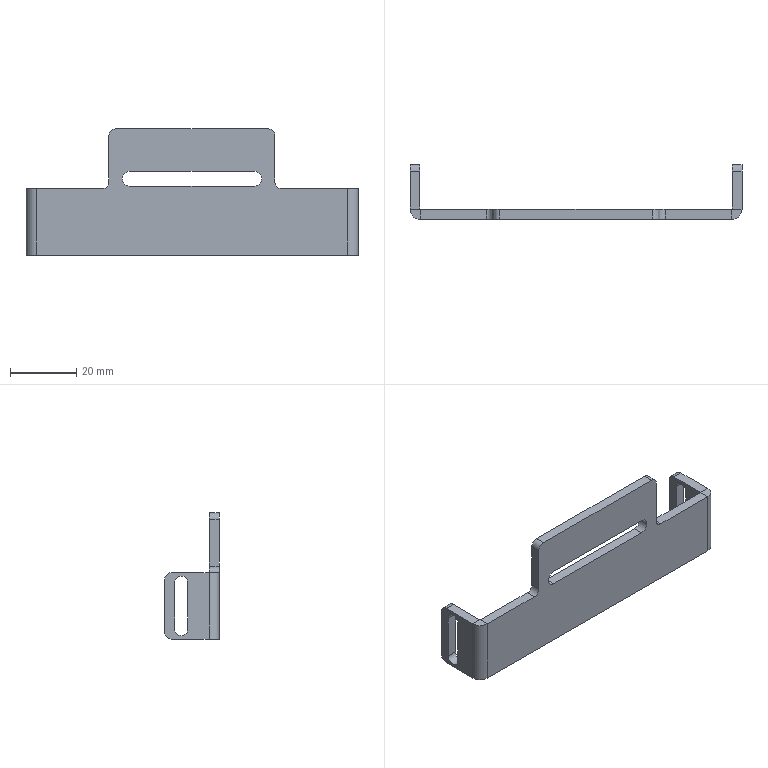Part | STEP file | 1 solid | 48 faces | box 100 x 16.5 x 38 mm | volume 9262 mm3 | plane 28 | cylinder 20 | commonest cylinder face diameters 4 x14 0.2 x2 4.5 x2 6.2 x2